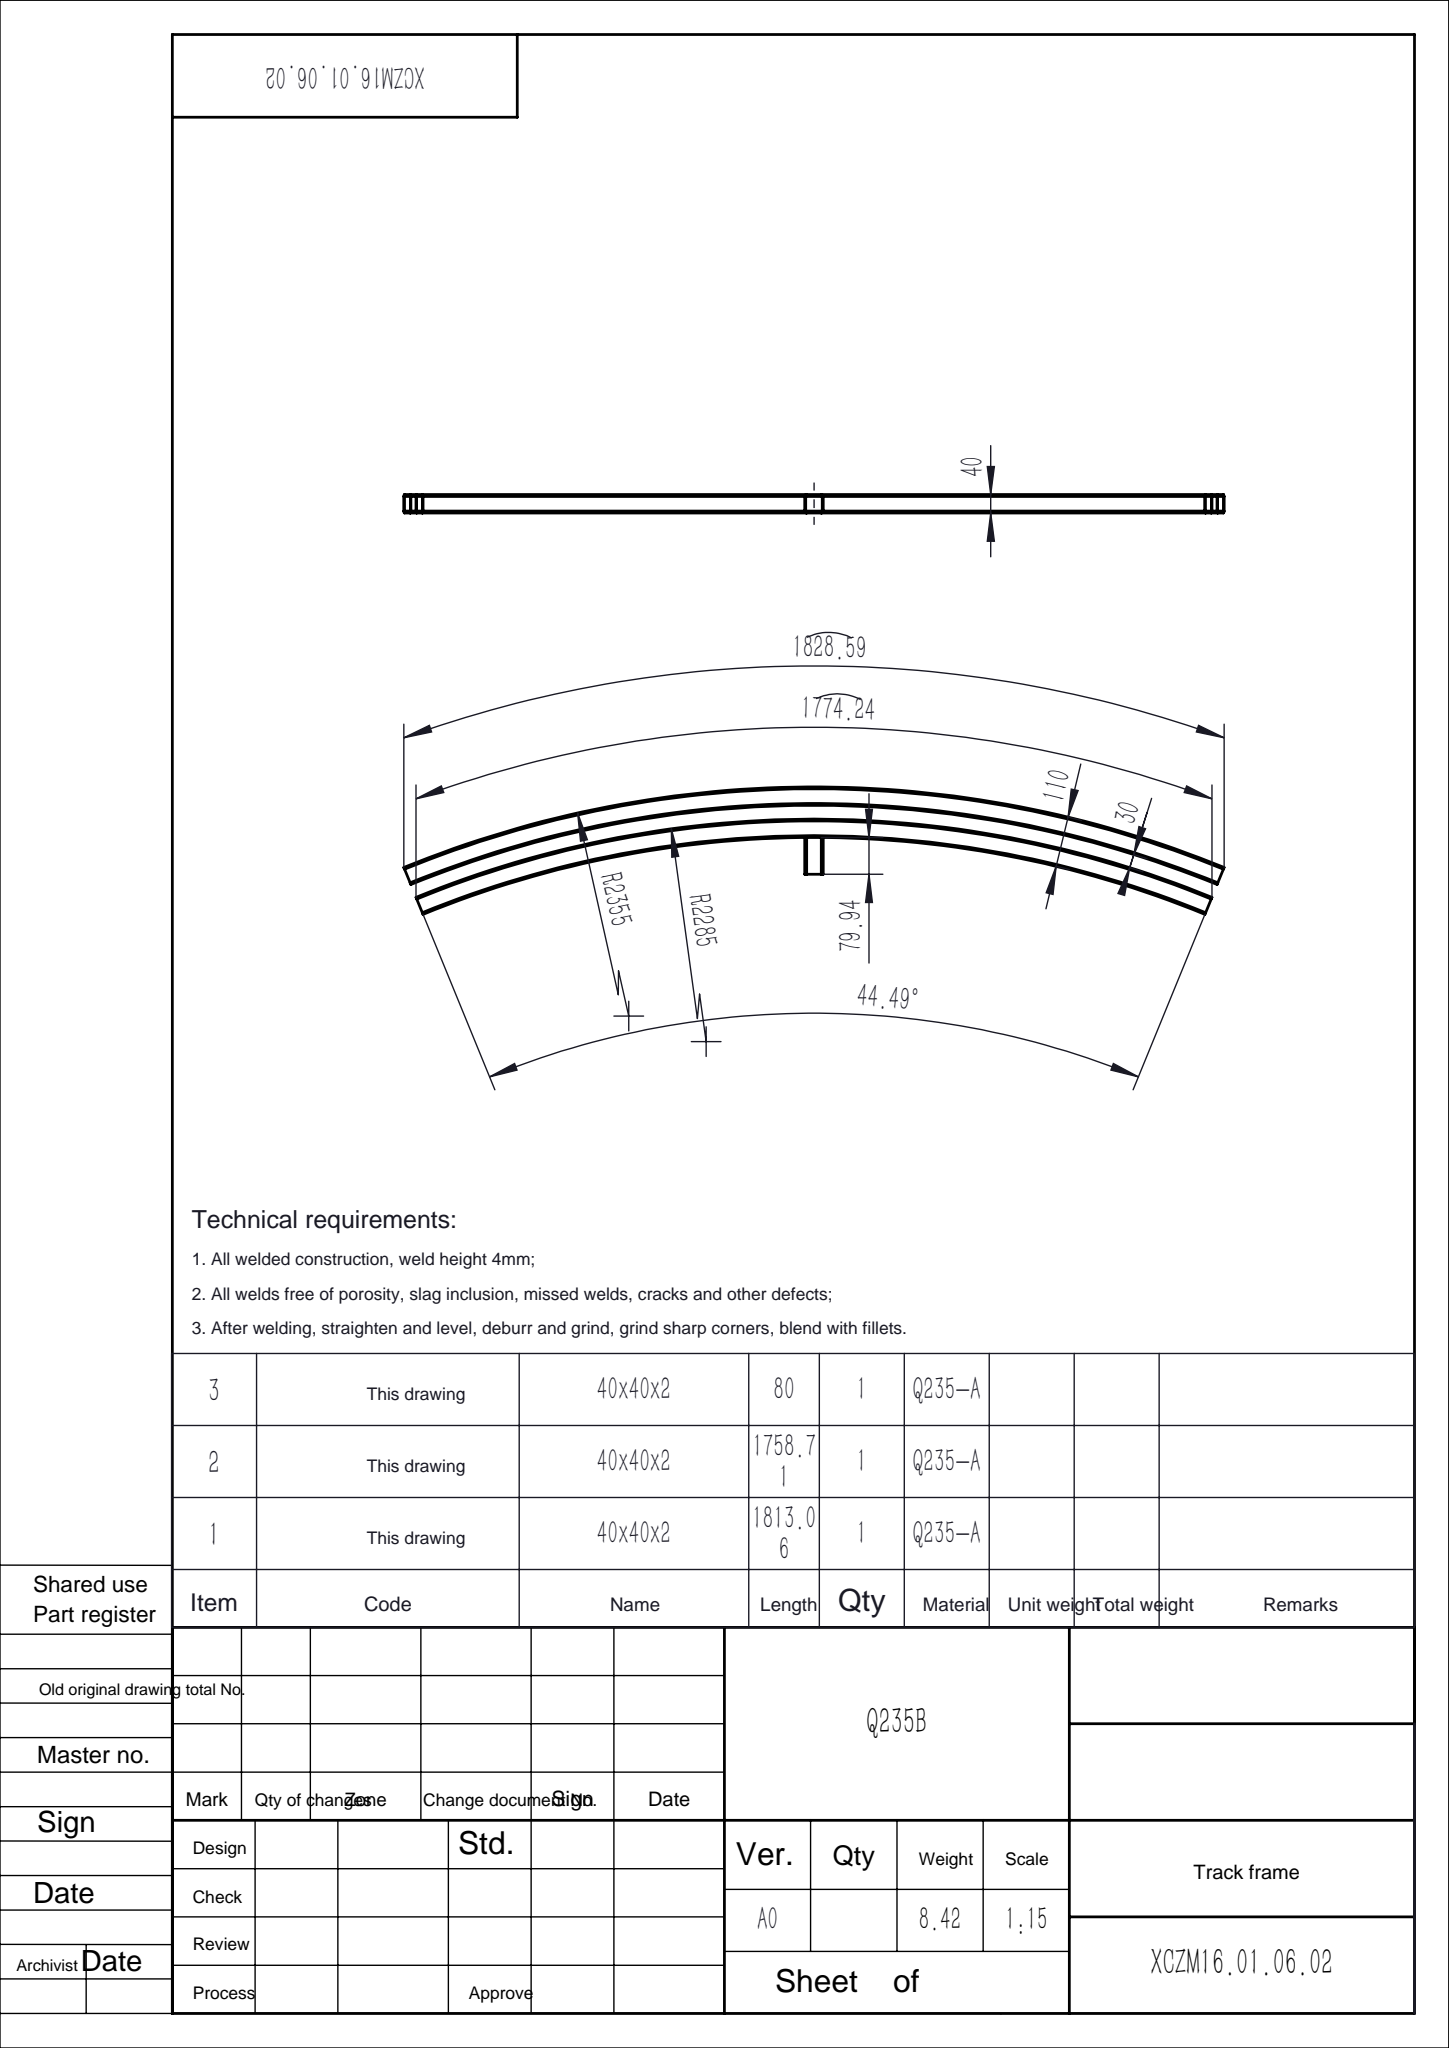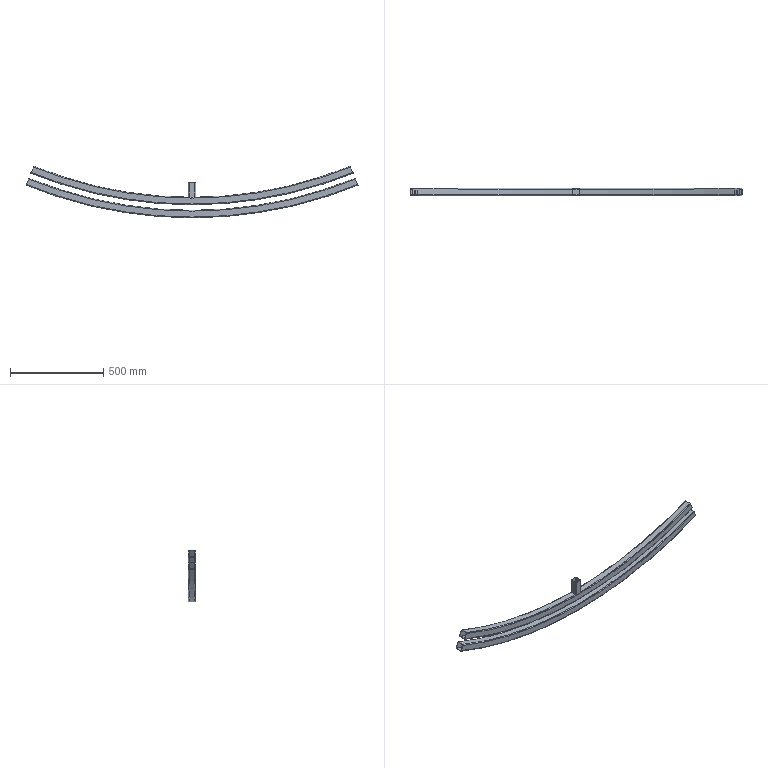Part | SolidWorks | features WeldCornerFeat 1, WeldMemberFeat 1, WeldmentFeature 1 | 3 solids | 54 faces | box 1783 x 40 x 277.077 mm | volume 1072506 mm3 | plane 21 | cylinder 17 | torus 16 | commonest cylinder face diameters 4 x4 8 x4 4490 x2 4494 x1 4566 x1 4570 x1